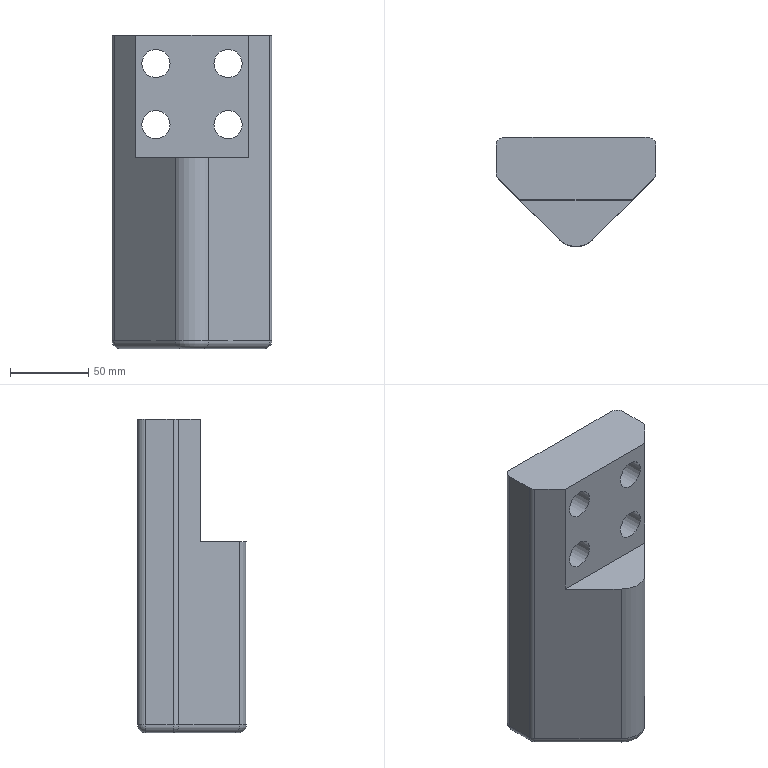Part | NX | features UB-7 2 | 1 solid | 36 faces | box 102 x 69.645 x 200 mm | volume 855541 mm3 | cylinder 18 | plane 13 | sphere 4 | torus 1 | commonest cylinder face diameters 10 x9 18 x4 26 x4 30 x1
STEP:
#1=CARTESIAN_POINT('',(3357.129,-625.444,973.716));
#2=VERTEX_POINT('',#1);
#3=CARTESIAN_POINT('',(3343.452,-639.122,973.716));
#4=VERTEX_POINT('',#3);
#5=CARTESIAN_POINT('',(3333.023,-649.551,973.716));
#6=DIRECTION('',(-0.7071,-0.7071,0.));
#7=VECTOR('',#6,1000.);
#8=LINE('',#5,#7);
#9=EDGE_CURVE('',#2,#4,#8,.T.);
#10=ORIENTED_EDGE('',*,*,#9,.F.);
#11=CARTESIAN_POINT('',(3358.594,-621.909,973.716));
#12=VERTEX_POINT('',#11);
#13=CARTESIAN_POINT('',(3353.594,-621.909,973.716));
#14=DIRECTION('',(0.,0.,-1.));
#15=DIRECTION('',(1.,0.,0.));
#16=AXIS2_PLACEMENT_3D('',#13,#14,#15);
#17=CIRCLE('',#16,5.);
#18=EDGE_CURVE('',#12,#2,#17,.T.);
#19=ORIENTED_EDGE('',*,*,#18,.F.);
#20=CARTESIAN_POINT('',(3358.594,-604.122,973.716));
#21=VERTEX_POINT('',#20);
#22=CARTESIAN_POINT('',(3358.594,-656.622,973.716));
#23=DIRECTION('',(0.,-1.,0.));
#24=VECTOR('',#23,1000.);
#25=LINE('',#22,#24);
#26=EDGE_CURVE('',#21,#12,#25,.T.);
#27=ORIENTED_EDGE('',*,*,#26,.F.);
#28=CARTESIAN_POINT('',(3353.594,-599.122,973.716));
#29=VERTEX_POINT('',#28);
#30=CARTESIAN_POINT('',(3353.594,-604.122,973.716));
#31=DIRECTION('',(0.,0.,-1.));
#32=DIRECTION('',(1.,0.,0.));
#33=AXIS2_PLACEMENT_3D('',#30,#31,#32);
#34=CIRCLE('',#33,5.);
#35=EDGE_CURVE('',#29,#21,#34,.T.);
#36=ORIENTED_EDGE('',*,*,#35,.F.);
#37=CARTESIAN_POINT('',(3331.979,-599.122,973.716));
#38=VERTEX_POINT('',#37);
#39=CARTESIAN_POINT('',(3325.523,-599.122,973.716));
#40=DIRECTION('',(-1.,0.,0.));
#41=VECTOR('',#40,1000.);
#42=LINE('',#39,#41);
#43=EDGE_CURVE('',#29,#38,#42,.T.);
#44=ORIENTED_EDGE('',*,*,#43,.T.);
#45=CARTESIAN_POINT('',(3261.594,-599.122,973.716));
#46=VERTEX_POINT('',#45);
#47=CARTESIAN_POINT('',(3325.523,-599.122,973.716));
#48=DIRECTION('',(-1.,0.,0.));
#49=VECTOR('',#48,1000.);
#50=LINE('',#47,#49);
#51=EDGE_CURVE('',#38,#46,#50,.T.);
#52=ORIENTED_EDGE('',*,*,#51,.T.);
#53=CARTESIAN_POINT('',(3256.594,-604.122,973.716));
#54=VERTEX_POINT('',#53);
#55=CARTESIAN_POINT('',(3261.594,-604.122,973.716));
#56=DIRECTION('',(0.,0.,-1.));
#57=DIRECTION('',(1.,0.,0.));
#58=AXIS2_PLACEMENT_3D('',#55,#56,#57);
#59=CIRCLE('',#58,5.);
#60=EDGE_CURVE('',#54,#46,#59,.T.);
#61=ORIENTED_EDGE('',*,*,#60,.F.);
#62=CARTESIAN_POINT('',(3256.594,-621.909,973.716));
#63=VERTEX_POINT('',#62);
#64=CARTESIAN_POINT('',(3256.594,-656.622,973.716));
#65=DIRECTION('',(0.,-1.,0.));
#66=VECTOR('',#65,1000.);
#67=LINE('',#64,#66);
#68=EDGE_CURVE('',#54,#63,#67,.T.);
#69=ORIENTED_EDGE('',*,*,#68,.T.);
#70=CARTESIAN_POINT('',(3258.058,-625.444,973.716));
#71=VERTEX_POINT('',#70);
#72=CARTESIAN_POINT('',(3261.594,-621.909,973.716));
#73=DIRECTION('',(0.,0.,-1.));
#74=DIRECTION('',(1.,0.,0.));
#75=AXIS2_PLACEMENT_3D('',#72,#73,#74);
#76=CIRCLE('',#75,5.);
#77=EDGE_CURVE('',#71,#63,#76,.T.);
#78=ORIENTED_EDGE('',*,*,#77,.F.);
#79=CARTESIAN_POINT('',(3271.736,-639.122,973.716));
#80=VERTEX_POINT('',#79);
#81=CARTESIAN_POINT('',(3297.165,-664.551,973.716));
#82=DIRECTION('',(0.7071,-0.7071,0.));
#83=VECTOR('',#82,1000.);
#84=LINE('',#81,#83);
#85=EDGE_CURVE('',#71,#80,#84,.T.);
#86=ORIENTED_EDGE('',*,*,#85,.T.);
#87=CARTESIAN_POINT('',(3307.594,-639.122,973.716));
#88=DIRECTION('',(1.,0.,0.));
#89=VECTOR('',#88,1000.);
#90=LINE('',#87,#89);
#91=EDGE_CURVE('',#80,#4,#90,.T.);
#92=ORIENTED_EDGE('',*,*,#91,.T.);
#93=EDGE_LOOP('',(#10,#19,#27,#36,#44,#52,#61,#69,#78,#86,#92));
#94=FACE_BOUND('',#93,.T.);
#95=CARTESIAN_POINT('',(3325.523,-642.051,973.716));
#96=DIRECTION('',(0.,0.,1.));
#97=DIRECTION('',(0.7071,0.7071,0.));
#98=AXIS2_PLACEMENT_3D('',#95,#96,#97);
#99=PLANE('',#98);
#100=ADVANCED_FACE('',(#94),#99,.T.);
#101=CARTESIAN_POINT('',(3258.058,-625.444,778.716));
#102=VERTEX_POINT('',#101);
#103=CARTESIAN_POINT('',(3258.058,-625.444,583.116));
#104=DIRECTION('',(0.,0.,1.));
#105=VECTOR('',#104,1000.);
#106=LINE('',#103,#105);
#107=EDGE_CURVE('',#102,#71,#106,.T.);
#108=ORIENTED_EDGE('',*,*,#107,.T.);
#109=ORIENTED_EDGE('',*,*,#77,.T.);
#110=CARTESIAN_POINT('',(3256.594,-621.909,778.716));
#111=VERTEX_POINT('',#110);
#112=CARTESIAN_POINT('',(3256.594,-621.909,938.716));
#113=DIRECTION('',(0.,0.,-1.));
#114=VECTOR('',#113,1000.);
#115=LINE('',#112,#114);
#116=EDGE_CURVE('',#63,#111,#115,.T.);
#117=ORIENTED_EDGE('',*,*,#116,.T.);
#118=CARTESIAN_POINT('',(3261.594,-621.909,778.716));
#119=DIRECTION('',(0.,0.,-1.));
#120=DIRECTION('',(1.,0.,0.));
#121=AXIS2_PLACEMENT_3D('',#118,#119,#120);
#122=CIRCLE('',#121,5.);
#123=EDGE_CURVE('',#102,#111,#122,.T.);
#124=ORIENTED_EDGE('',*,*,#123,.F.);
#125=EDGE_LOOP('',(#108,#109,#117,#124));
#126=FACE_BOUND('',#125,.T.);
#127=CARTESIAN_POINT('',(3261.594,-621.909,583.116));
#128=DIRECTION('',(0.,0.,1.));
#129=DIRECTION('',(-1.,0.,0.));
#130=AXIS2_PLACEMENT_3D('',#127,#128,#129);
#131=CYLINDRICAL_SURFACE('',#130,5.);
#132=ADVANCED_FACE('',(#126),#131,.T.);
#133=CARTESIAN_POINT('',(3358.594,-621.909,778.716));
#134=VERTEX_POINT('',#133);
#135=CARTESIAN_POINT('',(3358.594,-621.909,968.716));
#136=DIRECTION('',(0.,0.,1.));
#137=VECTOR('',#136,1000.);
#138=LINE('',#135,#137);
#139=EDGE_CURVE('',#134,#12,#138,.T.);
#140=ORIENTED_EDGE('',*,*,#139,.T.);
#141=ORIENTED_EDGE('',*,*,#18,.T.);
#142=CARTESIAN_POINT('',(3357.129,-625.444,778.716));
#143=VERTEX_POINT('',#142);
#144=CARTESIAN_POINT('',(3357.129,-625.444,943.716));
#145=DIRECTION('',(0.,0.,-1.));
#146=VECTOR('',#145,1000.);
#147=LINE('',#144,#146);
#148=EDGE_CURVE('',#2,#143,#147,.T.);
#149=ORIENTED_EDGE('',*,*,#148,.T.);
#150=CARTESIAN_POINT('',(3353.594,-621.909,778.716));
#151=DIRECTION('',(0.,0.,-1.));
#152=DIRECTION('',(1.,0.,0.));
#153=AXIS2_PLACEMENT_3D('',#150,#151,#152);
#154=CIRCLE('',#153,5.);
#155=EDGE_CURVE('',#134,#143,#154,.T.);
#156=ORIENTED_EDGE('',*,*,#155,.F.);
#157=EDGE_LOOP('',(#140,#141,#149,#156));
#158=FACE_BOUND('',#157,.T.);
#159=CARTESIAN_POINT('',(3353.594,-621.909,943.716));
#160=DIRECTION('',(0.,0.,1.));
#161=DIRECTION('',(-1.,0.,0.));
#162=AXIS2_PLACEMENT_3D('',#159,#160,#161);
#163=CYLINDRICAL_SURFACE('',#162,5.);
#164=ADVANCED_FACE('',(#158),#163,.T.);
#165=CARTESIAN_POINT('',(3353.594,-599.122,778.716));
#166=VERTEX_POINT('',#165);
#167=CARTESIAN_POINT('',(3353.594,-599.122,858.716));
#168=DIRECTION('',(0.,0.,1.));
#169=VECTOR('',#168,1000.);
#170=LINE('',#167,#169);
#171=EDGE_CURVE('',#166,#29,#170,.T.);
#172=ORIENTED_EDGE('',*,*,#171,.T.);
#173=ORIENTED_EDGE('',*,*,#35,.T.);
#174=CARTESIAN_POINT('',(3358.594,-604.122,778.716));
#175=VERTEX_POINT('',#174);
#176=CARTESIAN_POINT('',(3358.594,-604.122,938.716));
#177=DIRECTION('',(0.,0.,-1.));
#178=VECTOR('',#177,1000.);
#179=LINE('',#176,#178);
#180=EDGE_CURVE('',#21,#175,#179,.T.);
#181=ORIENTED_EDGE('',*,*,#180,.T.);
#182=CARTESIAN_POINT('',(3353.594,-604.122,778.716));
#183=DIRECTION('',(0.,0.,-1.));
#184=DIRECTION('',(1.,0.,0.));
#185=AXIS2_PLACEMENT_3D('',#182,#183,#184);
#186=CIRCLE('',#185,5.);
#187=EDGE_CURVE('',#166,#175,#186,.T.);
#188=ORIENTED_EDGE('',*,*,#187,.F.);
#189=EDGE_LOOP('',(#172,#173,#181,#188));
#190=FACE_BOUND('',#189,.T.);
#191=CARTESIAN_POINT('',(3353.594,-604.122,858.716));
#192=DIRECTION('',(0.,0.,1.));
#193=DIRECTION('',(-1.,0.,0.));
#194=AXIS2_PLACEMENT_3D('',#191,#192,#193);
#195=CYLINDRICAL_SURFACE('',#194,5.);
#196=ADVANCED_FACE('',(#190),#195,.T.);
#197=ORIENTED_EDGE('',*,*,#180,.F.);
#198=ORIENTED_EDGE('',*,*,#26,.T.);
#199=ORIENTED_EDGE('',*,*,#139,.F.);
#200=CARTESIAN_POINT('',(3358.594,-621.909,778.716));
#201=DIRECTION('',(0.,-1.,0.));
#202=VECTOR('',#201,1000.);
#203=LINE('',#200,#202);
#204=EDGE_CURVE('',#175,#134,#203,.T.);
#205=ORIENTED_EDGE('',*,*,#204,.F.);
#206=EDGE_LOOP('',(#197,#198,#199,#205));
#207=FACE_BOUND('',#206,.T.);
#208=CARTESIAN_POINT('',(3358.594,-656.622,938.716));
#209=DIRECTION('',(1.,0.,0.));
#210=DIRECTION('',(0.,0.,1.));
#211=AXIS2_PLACEMENT_3D('',#208,#209,#210);
#212=PLANE('',#211);
#213=ADVANCED_FACE('',(#207),#212,.T.);
#214=CARTESIAN_POINT('',(3256.594,-604.122,778.716));
#215=VERTEX_POINT('',#214);
#216=CARTESIAN_POINT('',(3256.594,-604.122,968.716));
#217=DIRECTION('',(0.,0.,1.));
#218=VECTOR('',#217,1000.);
#219=LINE('',#216,#218);
#220=EDGE_CURVE('',#215,#54,#219,.T.);
#221=ORIENTED_EDGE('',*,*,#220,.T.);
#222=ORIENTED_EDGE('',*,*,#60,.T.);
#223=CARTESIAN_POINT('',(3261.594,-599.122,778.716));
#224=VERTEX_POINT('',#223);
#225=CARTESIAN_POINT('',(3261.594,-599.122,898.716));
#226=DIRECTION('',(0.,0.,-1.));
#227=VECTOR('',#226,1000.);
#228=LINE('',#225,#227);
#229=EDGE_CURVE('',#46,#224,#228,.T.);
#230=ORIENTED_EDGE('',*,*,#229,.T.);
#231=CARTESIAN_POINT('',(3261.594,-604.122,778.716));
#232=DIRECTION('',(0.,0.,-1.));
#233=DIRECTION('',(-1.,0.,0.));
#234=AXIS2_PLACEMENT_3D('',#231,#232,#233);
#235=CIRCLE('',#234,5.);
#236=EDGE_CURVE('',#215,#224,#235,.T.);
#237=ORIENTED_EDGE('',*,*,#236,.F.);
#238=EDGE_LOOP('',(#221,#222,#230,#237));
#239=FACE_BOUND('',#238,.T.);
#240=CARTESIAN_POINT('',(3261.594,-604.122,858.716));
#241=DIRECTION('',(0.,0.,-1.));
#242=DIRECTION('',(1.,0.,0.));
#243=AXIS2_PLACEMENT_3D('',#240,#241,#242);
#244=CYLINDRICAL_SURFACE('',#243,5.);
#245=ADVANCED_FACE('',(#239),#244,.T.);
#246=CARTESIAN_POINT('',(3297.594,-599.122,955.716));
#247=VERTEX_POINT('',#246);
#248=CARTESIAN_POINT('',(3284.594,-599.122,955.716));
#249=DIRECTION('',(0.,-1.,0.));
#250=DIRECTION('',(1.,0.,0.));
#251=AXIS2_PLACEMENT_3D('',#248,#249,#250);
#252=CIRCLE('',#251,13.);
#253=EDGE_CURVE('',#247,#247,#252,.T.);
#254=ORIENTED_EDGE('',*,*,#253,.T.);
#255=EDGE_LOOP('',(#254));
#256=FACE_BOUND('',#255,.T.);
#257=CARTESIAN_POINT('',(3343.594,-599.122,916.716));
#258=VERTEX_POINT('',#257);
#259=CARTESIAN_POINT('',(3330.594,-599.122,916.716));
#260=DIRECTION('',(0.,-1.,0.));
#261=DIRECTION('',(1.,0.,0.));
#262=AXIS2_PLACEMENT_3D('',#259,#260,#261);
#263=CIRCLE('',#262,13.);
#264=EDGE_CURVE('',#258,#258,#263,.T.);
#265=ORIENTED_EDGE('',*,*,#264,.T.);
#266=EDGE_LOOP('',(#265));
#267=FACE_BOUND('',#266,.T.);
#268=CARTESIAN_POINT('',(3297.594,-599.122,916.716));
#269=VERTEX_POINT('',#268);
#270=CARTESIAN_POINT('',(3284.594,-599.122,916.716));
#271=DIRECTION('',(0.,-1.,0.));
#272=DIRECTION('',(1.,0.,0.));
#273=AXIS2_PLACEMENT_3D('',#270,#271,#272);
#274=CIRCLE('',#273,13.);
#275=EDGE_CURVE('',#269,#269,#274,.T.);
#276=ORIENTED_EDGE('',*,*,#275,.T.);
#277=EDGE_LOOP('',(#276));
#278=FACE_BOUND('',#277,.T.);
#279=CARTESIAN_POINT('',(3343.594,-599.122,955.716));
#280=VERTEX_POINT('',#279);
#281=CARTESIAN_POINT('',(3330.594,-599.122,955.716));
#282=DIRECTION('',(0.,-1.,0.));
#283=DIRECTION('',(1.,0.,0.));
#284=AXIS2_PLACEMENT_3D('',#281,#282,#283);
#285=CIRCLE('',#284,13.);
#286=EDGE_CURVE('',#280,#280,#285,.T.);
#287=ORIENTED_EDGE('',*,*,#286,.T.);
#288=EDGE_LOOP('',(#287));
#289=FACE_BOUND('',#288,.T.);
#290=ORIENTED_EDGE('',*,*,#229,.F.);
#291=ORIENTED_EDGE('',*,*,#51,.F.);
#292=ORIENTED_EDGE('',*,*,#43,.F.);
#293=ORIENTED_EDGE('',*,*,#171,.F.);
#294=CARTESIAN_POINT('',(3353.594,-599.122,778.716));
#295=DIRECTION('',(1.,0.,0.));
#296=VECTOR('',#295,1000.);
#297=LINE('',#294,#296);
#298=EDGE_CURVE('',#224,#166,#297,.T.);
#299=ORIENTED_EDGE('',*,*,#298,.F.);
#300=EDGE_LOOP('',(#290,#291,#292,#293,#299));
#301=FACE_BOUND('',#300,.T.);
#302=CARTESIAN_POINT('',(4400.094,-599.122,858.716));
#303=DIRECTION('',(0.,1.,0.));
#304=DIRECTION('',(-1.,0.,0.));
#305=AXIS2_PLACEMENT_3D('',#302,#303,#304);
#306=PLANE('',#305);
#307=ADVANCED_FACE('',(#256,#267,#278,#289,#301),#306,.T.);
#308=CARTESIAN_POINT('',(3293.594,-639.122,955.716));
#309=VERTEX_POINT('',#308);
#310=CARTESIAN_POINT('',(3284.594,-639.122,955.716));
#311=DIRECTION('',(0.,-1.,0.));
#312=DIRECTION('',(1.,0.,0.));
#313=AXIS2_PLACEMENT_3D('',#310,#311,#312);
#314=CIRCLE('',#313,9.);
#315=EDGE_CURVE('',#309,#309,#314,.T.);
#316=ORIENTED_EDGE('',*,*,#315,.F.);
#317=EDGE_LOOP('',(#316));
#318=FACE_BOUND('',#317,.T.);
#319=CARTESIAN_POINT('',(3339.594,-639.122,916.716));
#320=VERTEX_POINT('',#319);
#321=CARTESIAN_POINT('',(3330.594,-639.122,916.716));
#322=DIRECTION('',(0.,-1.,0.));
#323=DIRECTION('',(1.,0.,0.));
#324=AXIS2_PLACEMENT_3D('',#321,#322,#323);
#325=CIRCLE('',#324,9.);
#326=EDGE_CURVE('',#320,#320,#325,.T.);
#327=ORIENTED_EDGE('',*,*,#326,.F.);
#328=EDGE_LOOP('',(#327));
#329=FACE_BOUND('',#328,.T.);
#330=CARTESIAN_POINT('',(3293.594,-639.122,916.716));
#331=VERTEX_POINT('',#330);
#332=CARTESIAN_POINT('',(3284.594,-639.122,916.716));
#333=DIRECTION('',(0.,-1.,0.));
#334=DIRECTION('',(1.,0.,0.));
#335=AXIS2_PLACEMENT_3D('',#332,#333,#334);
#336=CIRCLE('',#335,9.);
#337=EDGE_CURVE('',#331,#331,#336,.T.);
#338=ORIENTED_EDGE('',*,*,#337,.F.);
#339=EDGE_LOOP('',(#338));
#340=FACE_BOUND('',#339,.T.);
#341=CARTESIAN_POINT('',(3339.594,-639.122,955.716));
#342=VERTEX_POINT('',#341);
#343=CARTESIAN_POINT('',(3330.594,-639.122,955.716));
#344=DIRECTION('',(0.,-1.,0.));
#345=DIRECTION('',(1.,0.,0.));
#346=AXIS2_PLACEMENT_3D('',#343,#344,#345);
#347=CIRCLE('',#346,9.);
#348=EDGE_CURVE('',#342,#342,#347,.T.);
#349=ORIENTED_EDGE('',*,*,#348,.F.);
#350=EDGE_LOOP('',(#349));
#351=FACE_BOUND('',#350,.T.);
#352=CARTESIAN_POINT('',(3343.452,-639.122,895.716));
#353=VERTEX_POINT('',#352);
#354=CARTESIAN_POINT('',(3343.452,-639.122,943.716));
#355=DIRECTION('',(0.,0.,1.));
#356=VECTOR('',#355,1000.);
#357=LINE('',#354,#356);
#358=EDGE_CURVE('',#353,#4,#357,.T.);
#359=ORIENTED_EDGE('',*,*,#358,.T.);
#360=ORIENTED_EDGE('',*,*,#91,.F.);
#361=CARTESIAN_POINT('',(3271.736,-639.122,895.716));
#362=VERTEX_POINT('',#361);
#363=CARTESIAN_POINT('',(3271.736,-639.122,933.716));
#364=DIRECTION('',(0.,0.,1.));
#365=VECTOR('',#364,1000.);
#366=LINE('',#363,#365);
#367=EDGE_CURVE('',#362,#80,#366,.T.);
#368=ORIENTED_EDGE('',*,*,#367,.F.);
#369=CARTESIAN_POINT('',(3307.594,-639.122,895.716));
#370=DIRECTION('',(-1.,0.,0.));
#371=VECTOR('',#370,1000.);
#372=LINE('',#369,#371);
#373=EDGE_CURVE('',#353,#362,#372,.T.);
#374=ORIENTED_EDGE('',*,*,#373,.F.);
#375=EDGE_LOOP('',(#359,#360,#368,#374));
#376=FACE_BOUND('',#375,.T.);
#377=CARTESIAN_POINT('',(3307.594,-639.122,933.716));
#378=DIRECTION('',(0.,1.,0.));
#379=DIRECTION('',(-1.,0.,0.));
#380=AXIS2_PLACEMENT_3D('',#377,#378,#379);
#381=PLANE('',#380);
#382=ADVANCED_FACE('',(#318,#329,#340,#351,#376),#381,.F.);
#383=ORIENTED_EDGE('',*,*,#148,.F.);
#384=ORIENTED_EDGE('',*,*,#9,.T.);
#385=ORIENTED_EDGE('',*,*,#358,.F.);
#386=CARTESIAN_POINT('',(3318.201,-664.373,895.716));
#387=VERTEX_POINT('',#386);
#388=CARTESIAN_POINT('',(3333.023,-649.551,895.716));
#389=DIRECTION('',(0.7071,0.7071,0.));
#390=VECTOR('',#389,1000.);
#391=LINE('',#388,#390);
#392=EDGE_CURVE('',#387,#353,#391,.T.);
#393=ORIENTED_EDGE('',*,*,#392,.F.);
#394=CARTESIAN_POINT('',(3318.201,-664.373,778.716));
#395=VERTEX_POINT('',#394);
#396=CARTESIAN_POINT('',(3318.201,-664.373,943.716));
#397=DIRECTION('',(0.,0.,1.));
#398=VECTOR('',#397,1000.);
#399=LINE('',#396,#398);
#400=EDGE_CURVE('',#395,#387,#399,.T.);
#401=ORIENTED_EDGE('',*,*,#400,.F.);
#402=CARTESIAN_POINT('',(3333.023,-649.551,778.716));
#403=DIRECTION('',(-0.7071,-0.7071,0.));
#404=VECTOR('',#403,1000.);
#405=LINE('',#402,#404);
#406=EDGE_CURVE('',#143,#395,#405,.T.);
#407=ORIENTED_EDGE('',*,*,#406,.F.);
#408=EDGE_LOOP('',(#383,#384,#385,#393,#401,#407));
#409=FACE_BOUND('',#408,.T.);
#410=CARTESIAN_POINT('',(3333.023,-649.551,943.716));
#411=DIRECTION('',(-0.7071,0.7071,0.));
#412=DIRECTION('',(-0.7071,-0.7071,0.));
#413=AXIS2_PLACEMENT_3D('',#410,#411,#412);
#414=PLANE('',#413);
#415=ADVANCED_FACE('',(#409),#414,.F.);
#416=ORIENTED_EDGE('',*,*,#116,.F.);
#417=ORIENTED_EDGE('',*,*,#68,.F.);
#418=ORIENTED_EDGE('',*,*,#220,.F.);
#419=CARTESIAN_POINT('',(3256.594,-656.622,778.716));
#420=DIRECTION('',(0.,1.,0.));
#421=VECTOR('',#420,1000.);
#422=LINE('',#419,#421);
#423=EDGE_CURVE('',#111,#215,#422,.T.);
#424=ORIENTED_EDGE('',*,*,#423,.F.);
#425=EDGE_LOOP('',(#416,#417,#418,#424));
#426=FACE_BOUND('',#425,.T.);
#427=CARTESIAN_POINT('',(3256.594,-656.622,938.716));
#428=DIRECTION('',(-1.,0.,0.));
#429=DIRECTION('',(0.,0.,-1.));
#430=AXIS2_PLACEMENT_3D('',#427,#428,#429);
#431=PLANE('',#430);
#432=ADVANCED_FACE('',(#426),#431,.T.);
#433=ORIENTED_EDGE('',*,*,#367,.T.);
#434=ORIENTED_EDGE('',*,*,#85,.F.);
#435=ORIENTED_EDGE('',*,*,#107,.F.);
#436=CARTESIAN_POINT('',(3296.987,-664.373,778.716));
#437=VERTEX_POINT('',#436);
#438=CARTESIAN_POINT('',(3297.165,-664.551,778.716));
#439=DIRECTION('',(-0.7071,0.7071,0.));
#440=VECTOR('',#439,1000.);
#441=LINE('',#438,#440);
#442=EDGE_CURVE('',#437,#102,#441,.T.);
#443=ORIENTED_EDGE('',*,*,#442,.F.);
#444=CARTESIAN_POINT('',(3296.987,-664.373,895.716));
#445=VERTEX_POINT('',#444);
#446=CARTESIAN_POINT('',(3296.987,-664.373,583.116));
#447=DIRECTION('',(0.,0.,-1.));
#448=VECTOR('',#447,1000.);
#449=LINE('',#446,#448);
#450=EDGE_CURVE('',#445,#437,#449,.T.);
#451=ORIENTED_EDGE('',*,*,#450,.F.);
#452=CARTESIAN_POINT('',(3297.165,-664.551,895.716));
#453=DIRECTION('',(0.7071,-0.7071,0.));
#454=VECTOR('',#453,1000.);
#455=LINE('',#452,#454);
#456=EDGE_CURVE('',#362,#445,#455,.T.);
#457=ORIENTED_EDGE('',*,*,#456,.F.);
#458=EDGE_LOOP('',(#433,#434,#435,#443,#451,#457));
#459=FACE_BOUND('',#458,.T.);
#460=CARTESIAN_POINT('',(3297.165,-664.551,583.116));
#461=DIRECTION('',(-0.7071,-0.7071,0.));
#462=DIRECTION('',(0.,0.,1.));
#463=AXIS2_PLACEMENT_3D('',#460,#461,#462);
#464=PLANE('',#463);
#465=ADVANCED_FACE('',(#459),#464,.T.);
#466=ORIENTED_EDGE('',*,*,#392,.T.);
#467=ORIENTED_EDGE('',*,*,#373,.T.);
#468=ORIENTED_EDGE('',*,*,#456,.T.);
#469=CARTESIAN_POINT('',(3307.594,-653.767,895.716));
#470=DIRECTION('',(0.,0.,-1.));
#471=DIRECTION('',(-1.,0.,0.));
#472=AXIS2_PLACEMENT_3D('',#469,#470,#471);
#473=CIRCLE('',#472,15.);
#474=EDGE_CURVE('',#387,#445,#473,.T.);
#475=ORIENTED_EDGE('',*,*,#474,.F.);
#476=EDGE_LOOP('',(#466,#467,#468,#475));
#477=FACE_BOUND('',#476,.T.);
#478=CARTESIAN_POINT('',(3307.594,-651.622,895.716));
#479=DIRECTION('',(0.,0.,-1.));
#480=DIRECTION('',(1.,0.,0.));
#481=AXIS2_PLACEMENT_3D('',#478,#479,#480);
#482=PLANE('',#481);
#483=ADVANCED_FACE('',(#477),#482,.F.);
#484=CARTESIAN_POINT('',(3314.665,-660.838,773.716));
#485=VERTEX_POINT('',#484);
#486=CARTESIAN_POINT('',(3353.594,-621.909,773.716));
#487=VERTEX_POINT('',#486);
#488=CARTESIAN_POINT('',(3329.487,-646.015,773.716));
#489=DIRECTION('',(0.7071,0.7071,0.));
#490=VECTOR('',#489,1000.);
#491=LINE('',#488,#490);
#492=EDGE_CURVE('',#485,#487,#491,.T.);
#493=ORIENTED_EDGE('',*,*,#492,.F.);
#494=CARTESIAN_POINT('',(3300.523,-660.838,773.716));
#495=VERTEX_POINT('',#494);
#496=CARTESIAN_POINT('',(3307.594,-653.767,773.716));
#497=DIRECTION('',(0.,0.,1.));
#498=DIRECTION('',(1.,0.,0.));
#499=AXIS2_PLACEMENT_3D('',#496,#497,#498);
#500=CIRCLE('',#499,10.);
#501=EDGE_CURVE('',#495,#485,#500,.T.);
#502=ORIENTED_EDGE('',*,*,#501,.F.);
#503=CARTESIAN_POINT('',(3261.594,-621.909,773.716));
#504=VERTEX_POINT('',#503);
#505=CARTESIAN_POINT('',(3303.629,-663.944,773.716));
#506=DIRECTION('',(0.7071,-0.7071,0.));
#507=VECTOR('',#506,1000.);
#508=LINE('',#505,#507);
#509=EDGE_CURVE('',#504,#495,#508,.T.);
#510=ORIENTED_EDGE('',*,*,#509,.F.);
#511=CARTESIAN_POINT('',(3261.594,-604.122,773.716));
#512=VERTEX_POINT('',#511);
#513=CARTESIAN_POINT('',(3261.594,-642.051,773.716));
#514=DIRECTION('',(0.,-1.,0.));
#515=VECTOR('',#514,1000.);
#516=LINE('',#513,#515);
#517=EDGE_CURVE('',#512,#504,#516,.T.);
#518=ORIENTED_EDGE('',*,*,#517,.F.);
#519=CARTESIAN_POINT('',(3353.594,-604.122,773.716));
#520=VERTEX_POINT('',#519);
#521=CARTESIAN_POINT('',(3261.594,-604.122,773.716));
#522=DIRECTION('',(-1.,0.,0.));
#523=VECTOR('',#522,1000.);
#524=LINE('',#521,#523);
#525=EDGE_CURVE('',#520,#512,#524,.T.);
#526=ORIENTED_EDGE('',*,*,#525,.F.);
#527=CARTESIAN_POINT('',(3353.594,-609.122,773.716));
#528=DIRECTION('',(0.,1.,0.));
#529=VECTOR('',#528,1000.);
#530=LINE('',#527,#529);
#531=EDGE_CURVE('',#487,#520,#530,.T.);
#532=ORIENTED_EDGE('',*,*,#531,.F.);
#533=EDGE_LOOP('',(#493,#502,#510,#518,#526,#532));
#534=FACE_BOUND('',#533,.T.);
#535=CARTESIAN_POINT('',(3325.523,-642.051,773.716));
#536=DIRECTION('',(0.,0.,1.));
#537=DIRECTION('',(0.7071,0.7071,0.));
#538=AXIS2_PLACEMENT_3D('',#535,#536,#537);
#539=PLANE('',#538);
#540=ADVANCED_FACE('',(#534),#539,.F.);
#541=ORIENTED_EDGE('',*,*,#400,.T.);
#542=ORIENTED_EDGE('',*,*,#474,.T.);
#543=ORIENTED_EDGE('',*,*,#450,.T.);
#544=CARTESIAN_POINT('',(3307.594,-653.767,778.716));
#545=DIRECTION('',(0.,0.,-1.));
#546=DIRECTION('',(1.,0.,0.));
#547=AXIS2_PLACEMENT_3D('',#544,#545,#546);
#548=CIRCLE('',#547,15.);
#549=EDGE_CURVE('',#395,#437,#548,.T.);
#550=ORIENTED_EDGE('',*,*,#549,.F.);
#551=EDGE_LOOP('',(#541,#542,#543,#550));
#552=FACE_BOUND('',#551,.T.);
#553=CARTESIAN_POINT('',(3307.594,-653.767,583.116));
#554=DIRECTION('',(0.,0.,1.));
#555=DIRECTION('',(-1.,0.,0.));
#556=AXIS2_PLACEMENT_3D('',#553,#554,#555);
#557=CYLINDRICAL_SURFACE('',#556,15.);
#558=ADVANCED_FACE('',(#552),#557,.T.);
#559=CARTESIAN_POINT('',(3261.594,-621.909,778.716));
#560=DIRECTION('',(0.,-1.,0.));
#561=DIRECTION('',(0.,0.,-1.));
#562=AXIS2_PLACEMENT_3D('',#559,#560,#561);
#563=CIRCLE('',#562,5.);
#564=EDGE_CURVE('',#111,#504,#563,.T.);
#565=ORIENTED_EDGE('',*,*,#564,.T.);
#566=CARTESIAN_POINT('',(3261.594,-621.909,778.716));
#567=DIRECTION('',(-0.7071,0.7071,0.));
#568=DIRECTION('',(-0.7071,-0.7071,0.));
#569=AXIS2_PLACEMENT_3D('',#566,#567,#568);
#570=CIRCLE('',#569,5.);
#571=EDGE_CURVE('',#504,#102,#570,.T.);
#572=ORIENTED_EDGE('',*,*,#571,.T.);
#573=ORIENTED_EDGE('',*,*,#123,.T.);
#574=EDGE_LOOP('',(#565,#572,#573));
#575=FACE_BOUND('',#574,.T.);
#576=CARTESIAN_POINT('',(3261.594,-621.909,778.716));
#577=DIRECTION('',(0.,0.,1.));
#578=DIRECTION('',(-1.,0.,0.));
#579=AXIS2_PLACEMENT_3D('',#576,#577,#578);
#580=SPHERICAL_SURFACE('',#579,5.);
#581=ADVANCED_FACE('',(#575),#580,.T.);
#582=ORIENTED_EDGE('',*,*,#571,.F.);
#583=ORIENTED_EDGE('',*,*,#509,.T.);
#584=CARTESIAN_POINT('',(3300.523,-660.838,778.716));
#585=DIRECTION('',(-0.7071,0.7071,0.));
#586=DIRECTION('',(-0.7071,-0.7071,0.));
#587=AXIS2_PLACEMENT_3D('',#584,#585,#586);
#588=CIRCLE('',#587,5.);
#589=EDGE_CURVE('',#495,#437,#588,.T.);
#590=ORIENTED_EDGE('',*,*,#589,.T.);
#591=ORIENTED_EDGE('',*,*,#442,.T.);
#592=EDGE_LOOP('',(#582,#583,#590,#591));
#593=FACE_BOUND('',#592,.T.);
#594=CARTESIAN_POINT('',(3300.701,-661.015,778.716));
#595=DIRECTION('',(0.7071,-0.7071,0.));
#596=DIRECTION('',(0.7071,0.7071,0.));
#597=AXIS2_PLACEMENT_3D('',#594,#595,#596);
#598=CYLINDRICAL_SURFACE('',#597,5.);
#599=ADVANCED_FACE('',(#593),#598,.T.);
#600=ORIENTED_EDGE('',*,*,#564,.F.);
#601=ORIENTED_EDGE('',*,*,#423,.T.);
#602=CARTESIAN_POINT('',(3261.594,-604.122,778.716));
#603=DIRECTION('',(0.,-1.,0.));
#604=DIRECTION('',(0.,0.,-1.));
#605=AXIS2_PLACEMENT_3D('',#602,#603,#604);
#606=CIRCLE('',#605,5.);
#607=EDGE_CURVE('',#215,#512,#606,.T.);
#608=ORIENTED_EDGE('',*,*,#607,.T.);
#609=ORIENTED_EDGE('',*,*,#517,.T.);
#610=EDGE_LOOP('',(#600,#601,#608,#609));
#611=FACE_BOUND('',#610,.T.);
#612=CARTESIAN_POINT('',(3261.594,-642.051,778.716));
#613=DIRECTION('',(0.,1.,0.));
#614=DIRECTION('',(0.,0.,1.));
#615=AXIS2_PLACEMENT_3D('',#612,#613,#614);
#616=CYLINDRICAL_SURFACE('',#615,5.);
#617=ADVANCED_FACE('',(#611),#616,.T.);
#618=ORIENTED_EDGE('',*,*,#589,.F.);
#619=ORIENTED_EDGE('',*,*,#501,.T.);
#620=CARTESIAN_POINT('',(3314.665,-660.838,778.716));
#621=DIRECTION('',(-0.7071,-0.7071,0.));
#622=DIRECTION('',(-0.7071,0.7071,0.));
#623=AXIS2_PLACEMENT_3D('',#620,#621,#622);
#624=CIRCLE('',#623,5.);
#625=EDGE_CURVE('',#485,#395,#624,.T.);
#626=ORIENTED_EDGE('',*,*,#625,.T.);
#627=ORIENTED_EDGE('',*,*,#549,.T.);
#628=EDGE_LOOP('',(#618,#619,#626,#627));
#629=FACE_BOUND('',#628,.T.);
#630=CARTESIAN_POINT('',(3307.594,-653.767,778.716));
#631=DIRECTION('',(0.,0.,1.));
#632=DIRECTION('',(-1.,0.,0.));
#633=AXIS2_PLACEMENT_3D('',#630,#631,#632);
#634=TOROIDAL_SURFACE('',#633,10.,5.);
#635=ADVANCED_FACE('',(#629),#634,.T.);
#636=ORIENTED_EDGE('',*,*,#236,.T.);
#637=CARTESIAN_POINT('',(3261.594,-604.122,778.716));
#638=DIRECTION('',(-1.,0.,0.));
#639=DIRECTION('',(0.,-1.,0.));
#640=AXIS2_PLACEMENT_3D('',#637,#638,#639);
#641=CIRCLE('',#640,5.);
#642=EDGE_CURVE('',#224,#512,#641,.T.);
#643=ORIENTED_EDGE('',*,*,#642,.T.);
#644=ORIENTED_EDGE('',*,*,#607,.F.);
#645=EDGE_LOOP('',(#636,#643,#644));
#646=FACE_BOUND('',#645,.T.);
#647=CARTESIAN_POINT('',(3261.594,-604.122,778.716));
#648=DIRECTION('',(0.,0.,1.));
#649=DIRECTION('',(-1.,0.,0.));
#650=AXIS2_PLACEMENT_3D('',#647,#648,#649);
#651=SPHERICAL_SURFACE('',#650,5.);
#652=ADVANCED_FACE('',(#646),#651,.T.);
#653=ORIENTED_EDGE('',*,*,#625,.F.);
#654=ORIENTED_EDGE('',*,*,#492,.T.);
#655=CARTESIAN_POINT('',(3353.594,-621.909,778.716));
#656=DIRECTION('',(-0.7071,-0.7071,0.));
#657=DIRECTION('',(-0.7071,0.7071,0.));
#658=AXIS2_PLACEMENT_3D('',#655,#656,#657);
#659=CIRCLE('',#658,5.);
#660=EDGE_CURVE('',#487,#143,#659,.T.);
#661=ORIENTED_EDGE('',*,*,#660,.T.);
#662=ORIENTED_EDGE('',*,*,#406,.T.);
#663=EDGE_LOOP('',(#653,#654,#661,#662));
#664=FACE_BOUND('',#663,.T.);
#665=CARTESIAN_POINT('',(3329.487,-646.015,778.716));
#666=DIRECTION('',(-0.7071,-0.7071,0.));
#667=DIRECTION('',(0.7071,-0.7071,0.));
#668=AXIS2_PLACEMENT_3D('',#665,#666,#667);
#669=CYLINDRICAL_SURFACE('',#668,5.);
#670=ADVANCED_FACE('',(#664),#669,.T.);
#671=ORIENTED_EDGE('',*,*,#642,.F.);
#672=ORIENTED_EDGE('',*,*,#298,.T.);
#673=CARTESIAN_POINT('',(3353.594,-604.122,778.716));
#674=DIRECTION('',(-1.,0.,0.));
#675=DIRECTION('',(0.,-1.,0.));
#676=AXIS2_PLACEMENT_3D('',#673,#674,#675);
#677=CIRCLE('',#676,5.);
#678=EDGE_CURVE('',#166,#520,#677,.T.);
#679=ORIENTED_EDGE('',*,*,#678,.T.);
#680=ORIENTED_EDGE('',*,*,#525,.T.);
#681=EDGE_LOOP('',(#671,#672,#679,#680));
#682=FACE_BOUND('',#681,.T.);
#683=CARTESIAN_POINT('',(3325.523,-604.122,778.716));
#684=DIRECTION('',(1.,0.,0.));
#685=DIRECTION('',(0.,1.,0.));
#686=AXIS2_PLACEMENT_3D('',#683,#684,#685);
#687=CYLINDRICAL_SURFACE('',#686,5.);
#688=ADVANCED_FACE('',(#682),#687,.T.);
#689=ORIENTED_EDGE('',*,*,#660,.F.);
#690=CARTESIAN_POINT('',(3353.594,-621.909,778.716));
#691=DIRECTION('',(0.,-1.,0.));
#692=DIRECTION('',(0.,0.,1.));
#693=AXIS2_PLACEMENT_3D('',#690,#691,#692);
#694=CIRCLE('',#693,5.);
#695=EDGE_CURVE('',#487,#134,#694,.T.);
#696=ORIENTED_EDGE('',*,*,#695,.T.);
#697=ORIENTED_EDGE('',*,*,#155,.T.);
#698=EDGE_LOOP('',(#689,#696,#697));
#699=FACE_BOUND('',#698,.T.);
#700=CARTESIAN_POINT('',(3353.594,-621.909,778.716));
#701=DIRECTION('',(0.,0.,1.));
#702=DIRECTION('',(-1.,0.,0.));
#703=AXIS2_PLACEMENT_3D('',#700,#701,#702);
#704=SPHERICAL_SURFACE('',#703,5.);
#705=ADVANCED_FACE('',(#699),#704,.T.);
#706=ORIENTED_EDGE('',*,*,#187,.T.);
#707=CARTESIAN_POINT('',(3353.594,-604.122,778.716));
#708=DIRECTION('',(0.,1.,0.));
#709=DIRECTION('',(0.,0.,1.));
#710=AXIS2_PLACEMENT_3D('',#707,#708,#709);
#711=CIRCLE('',#710,5.);
#712=EDGE_CURVE('',#175,#520,#711,.T.);
#713=ORIENTED_EDGE('',*,*,#712,.T.);
#714=ORIENTED_EDGE('',*,*,#678,.F.);
#715=EDGE_LOOP('',(#706,#713,#714));
#716=FACE_BOUND('',#715,.T.);
#717=CARTESIAN_POINT('',(3353.594,-604.122,778.716));
#718=DIRECTION('',(0.,0.,1.));
#719=DIRECTION('',(-1.,0.,0.));
#720=AXIS2_PLACEMENT_3D('',#717,#718,#719);
#721=SPHERICAL_SURFACE('',#720,5.);
#722=ADVANCED_FACE('',(#716),#721,.T.);
#723=ORIENTED_EDGE('',*,*,#695,.F.);
#724=ORIENTED_EDGE('',*,*,#531,.T.);
#725=ORIENTED_EDGE('',*,*,#712,.F.);
#726=ORIENTED_EDGE('',*,*,#204,.T.);
#727=EDGE_LOOP('',(#723,#724,#725,#726));
#728=FACE_BOUND('',#727,.T.);
#729=CARTESIAN_POINT('',(3353.594,-642.051,778.716));
#730=DIRECTION('',(0.,-1.,0.));
#731=DIRECTION('',(0.,0.,-1.));
#732=AXIS2_PLACEMENT_3D('',#729,#730,#731);
#733=CYLINDRICAL_SURFACE('',#732,5.);
#734=ADVANCED_FACE('',(#728),#733,.T.);
#735=CARTESIAN_POINT('',(3339.594,-618.122,955.716));
#736=VERTEX_POINT('',#735);
#737=CARTESIAN_POINT('',(3330.594,-618.122,955.716));
#738=DIRECTION('',(0.,-1.,0.));
#739=DIRECTION('',(1.,0.,0.));
#740=AXIS2_PLACEMENT_3D('',#737,#738,#739);
#741=CIRCLE('',#740,9.);
#742=EDGE_CURVE('',#736,#736,#741,.T.);
#743=ORIENTED_EDGE('',*,*,#742,.F.);
#744=EDGE_LOOP('',(#743));
#745=FACE_BOUND('',#744,.T.);
#746=ORIENTED_EDGE('',*,*,#348,.T.);
#747=EDGE_LOOP('',(#746));
#748=FACE_BOUND('',#747,.T.);
#749=CARTESIAN_POINT('',(3330.594,-640.122,955.716));
#750=DIRECTION('',(0.,1.,0.));
#751=DIRECTION('',(0.,0.,1.));
#752=AXIS2_PLACEMENT_3D('',#749,#750,#751);
#753=CYLINDRICAL_SURFACE('',#752,9.);
#754=ADVANCED_FACE('',(#745,#748),#753,.F.);
#755=ORIENTED_EDGE('',*,*,#286,.F.);
#756=EDGE_LOOP('',(#755));
#757=FACE_BOUND('',#756,.T.);
#758=CARTESIAN_POINT('',(3317.594,-618.122,955.716));
#759=VERTEX_POINT('',#758);
#760=CARTESIAN_POINT('',(3330.594,-618.122,955.716));
#761=DIRECTION('',(0.,1.,0.));
#762=DIRECTION('',(-1.,0.,0.));
#763=AXIS2_PLACEMENT_3D('',#760,#761,#762);
#764=CIRCLE('',#763,13.);
#765=EDGE_CURVE('',#759,#759,#764,.T.);
#766=ORIENTED_EDGE('',*,*,#765,.F.);
#767=EDGE_LOOP('',(#766));
#768=FACE_BOUND('',#767,.T.);
#769=CARTESIAN_POINT('',(3330.594,-618.122,955.716));
#770=DIRECTION('',(0.,1.,0.));
#771=DIRECTION('',(0.,0.,1.));
#772=AXIS2_PLACEMENT_3D('',#769,#770,#771);
#773=CYLINDRICAL_SURFACE('',#772,13.);
#774=ADVANCED_FACE('',(#757,#768),#773,.F.);
#775=ORIENTED_EDGE('',*,*,#742,.T.);
#776=EDGE_LOOP('',(#775));
#777=FACE_BOUND('',#776,.T.);
#778=ORIENTED_EDGE('',*,*,#765,.T.);
#779=EDGE_LOOP('',(#778));
#780=FACE_BOUND('',#779,.T.);
#781=CARTESIAN_POINT('',(3330.594,-618.122,955.716));
#782=DIRECTION('',(0.,1.,0.));
#783=DIRECTION('',(-1.,0.,0.));
#784=AXIS2_PLACEMENT_3D('',#781,#782,#783);
#785=PLANE('',#784);
#786=ADVANCED_FACE('',(#777,#780),#785,.T.);
#787=CARTESIAN_POINT('',(3293.594,-618.122,916.716));
#788=VERTEX_POINT('',#787);
#789=CARTESIAN_POINT('',(3284.594,-618.122,916.716));
#790=DIRECTION('',(0.,-1.,0.));
#791=DIRECTION('',(1.,0.,0.));
#792=AXIS2_PLACEMENT_3D('',#789,#790,#791);
#793=CIRCLE('',#792,9.);
#794=EDGE_CURVE('',#788,#788,#793,.T.);
#795=ORIENTED_EDGE('',*,*,#794,.F.);
#796=EDGE_LOOP('',(#795));
#797=FACE_BOUND('',#796,.T.);
#798=ORIENTED_EDGE('',*,*,#337,.T.);
#799=EDGE_LOOP('',(#798));
#800=FACE_BOUND('',#799,.T.);
#801=CARTESIAN_POINT('',(3284.594,-640.122,916.716));
#802=DIRECTION('',(0.,1.,0.));
#803=DIRECTION('',(0.,0.,1.));
#804=AXIS2_PLACEMENT_3D('',#801,#802,#803);
#805=CYLINDRICAL_SURFACE('',#804,9.);
#806=ADVANCED_FACE('',(#797,#800),#805,.F.);
#807=ORIENTED_EDGE('',*,*,#275,.F.);
#808=EDGE_LOOP('',(#807));
#809=FACE_BOUND('',#808,.T.);
#810=CARTESIAN_POINT('',(3271.594,-618.122,916.716));
#811=VERTEX_POINT('',#810);
#812=CARTESIAN_POINT('',(3284.594,-618.122,916.716));
#813=DIRECTION('',(0.,1.,0.));
#814=DIRECTION('',(-1.,0.,0.));
#815=AXIS2_PLACEMENT_3D('',#812,#813,#814);
#816=CIRCLE('',#815,13.);
#817=EDGE_CURVE('',#811,#811,#816,.T.);
#818=ORIENTED_EDGE('',*,*,#817,.F.);
#819=EDGE_LOOP('',(#818));
#820=FACE_BOUND('',#819,.T.);
#821=CARTESIAN_POINT('',(3284.594,-618.122,916.716));
#822=DIRECTION('',(0.,1.,0.));
#823=DIRECTION('',(0.,0.,1.));
#824=AXIS2_PLACEMENT_3D('',#821,#822,#823);
#825=CYLINDRICAL_SURFACE('',#824,13.);
#826=ADVANCED_FACE('',(#809,#820),#825,.F.);
#827=ORIENTED_EDGE('',*,*,#794,.T.);
#828=EDGE_LOOP('',(#827));
#829=FACE_BOUND('',#828,.T.);
#830=ORIENTED_EDGE('',*,*,#817,.T.);
#831=EDGE_LOOP('',(#830));
#832=FACE_BOUND('',#831,.T.);
#833=CARTESIAN_POINT('',(3284.594,-618.122,916.716));
#834=DIRECTION('',(0.,1.,0.));
#835=DIRECTION('',(-1.,0.,0.));
#836=AXIS2_PLACEMENT_3D('',#833,#834,#835);
#837=PLANE('',#836);
#838=ADVANCED_FACE('',(#829,#832),#837,.T.);
#839=CARTESIAN_POINT('',(3339.594,-618.122,916.716));
#840=VERTEX_POINT('',#839);
#841=CARTESIAN_POINT('',(3330.594,-618.122,916.716));
#842=DIRECTION('',(0.,-1.,0.));
#843=DIRECTION('',(1.,0.,0.));
#844=AXIS2_PLACEMENT_3D('',#841,#842,#843);
#845=CIRCLE('',#844,9.);
#846=EDGE_CURVE('',#840,#840,#845,.T.);
#847=ORIENTED_EDGE('',*,*,#846,.F.);
#848=EDGE_LOOP('',(#847));
#849=FACE_BOUND('',#848,.T.);
#850=ORIENTED_EDGE('',*,*,#326,.T.);
#851=EDGE_LOOP('',(#850));
#852=FACE_BOUND('',#851,.T.);
#853=CARTESIAN_POINT('',(3330.594,-640.122,916.716));
#854=DIRECTION('',(0.,1.,0.));
#855=DIRECTION('',(0.,0.,1.));
#856=AXIS2_PLACEMENT_3D('',#853,#854,#855);
#857=CYLINDRICAL_SURFACE('',#856,9.);
#858=ADVANCED_FACE('',(#849,#852),#857,.F.);
#859=ORIENTED_EDGE('',*,*,#264,.F.);
#860=EDGE_LOOP('',(#859));
#861=FACE_BOUND('',#860,.T.);
#862=CARTESIAN_POINT('',(3317.594,-618.122,916.716));
#863=VERTEX_POINT('',#862);
#864=CARTESIAN_POINT('',(3330.594,-618.122,916.716));
#865=DIRECTION('',(0.,1.,0.));
#866=DIRECTION('',(-1.,0.,0.));
#867=AXIS2_PLACEMENT_3D('',#864,#865,#866);
#868=CIRCLE('',#867,13.);
#869=EDGE_CURVE('',#863,#863,#868,.T.);
#870=ORIENTED_EDGE('',*,*,#869,.F.);
#871=EDGE_LOOP('',(#870));
#872=FACE_BOUND('',#871,.T.);
#873=CARTESIAN_POINT('',(3330.594,-618.122,916.716));
#874=DIRECTION('',(0.,1.,0.));
#875=DIRECTION('',(0.,0.,1.));
#876=AXIS2_PLACEMENT_3D('',#873,#874,#875);
#877=CYLINDRICAL_SURFACE('',#876,13.);
#878=ADVANCED_FACE('',(#861,#872),#877,.F.);
#879=ORIENTED_EDGE('',*,*,#846,.T.);
#880=EDGE_LOOP('',(#879));
#881=FACE_BOUND('',#880,.T.);
#882=ORIENTED_EDGE('',*,*,#869,.T.);
#883=EDGE_LOOP('',(#882));
#884=FACE_BOUND('',#883,.T.);
#885=CARTESIAN_POINT('',(3330.594,-618.122,916.716));
#886=DIRECTION('',(0.,1.,0.));
#887=DIRECTION('',(-1.,0.,0.));
#888=AXIS2_PLACEMENT_3D('',#885,#886,#887);
#889=PLANE('',#888);
#890=ADVANCED_FACE('',(#881,#884),#889,.T.);
#891=CARTESIAN_POINT('',(3293.594,-618.122,955.716));
#892=VERTEX_POINT('',#891);
#893=CARTESIAN_POINT('',(3284.594,-618.122,955.716));
#894=DIRECTION('',(0.,-1.,0.));
#895=DIRECTION('',(1.,0.,0.));
#896=AXIS2_PLACEMENT_3D('',#893,#894,#895);
#897=CIRCLE('',#896,9.);
#898=EDGE_CURVE('',#892,#892,#897,.T.);
#899=ORIENTED_EDGE('',*,*,#898,.F.);
#900=EDGE_LOOP('',(#899));
#901=FACE_BOUND('',#900,.T.);
#902=ORIENTED_EDGE('',*,*,#315,.T.);
#903=EDGE_LOOP('',(#902));
#904=FACE_BOUND('',#903,.T.);
#905=CARTESIAN_POINT('',(3284.594,-640.122,955.716));
#906=DIRECTION('',(0.,1.,0.));
#907=DIRECTION('',(0.,0.,1.));
#908=AXIS2_PLACEMENT_3D('',#905,#906,#907);
#909=CYLINDRICAL_SURFACE('',#908,9.);
#910=ADVANCED_FACE('',(#901,#904),#909,.F.);
#911=ORIENTED_EDGE('',*,*,#253,.F.);
#912=EDGE_LOOP('',(#911));
#913=FACE_BOUND('',#912,.T.);
#914=CARTESIAN_POINT('',(3271.594,-618.122,955.716));
#915=VERTEX_POINT('',#914);
#916=CARTESIAN_POINT('',(3284.594,-618.122,955.716));
#917=DIRECTION('',(0.,1.,0.));
#918=DIRECTION('',(-1.,0.,0.));
#919=AXIS2_PLACEMENT_3D('',#916,#917,#918);
#920=CIRCLE('',#919,13.);
#921=EDGE_CURVE('',#915,#915,#920,.T.);
#922=ORIENTED_EDGE('',*,*,#921,.F.);
#923=EDGE_LOOP('',(#922));
#924=FACE_BOUND('',#923,.T.);
#925=CARTESIAN_POINT('',(3284.594,-618.122,955.716));
#926=DIRECTION('',(0.,1.,0.));
#927=DIRECTION('',(0.,0.,1.));
#928=AXIS2_PLACEMENT_3D('',#925,#926,#927);
#929=CYLINDRICAL_SURFACE('',#928,13.);
#930=ADVANCED_FACE('',(#913,#924),#929,.F.);
#931=ORIENTED_EDGE('',*,*,#898,.T.);
#932=EDGE_LOOP('',(#931));
#933=FACE_BOUND('',#932,.T.);
#934=ORIENTED_EDGE('',*,*,#921,.T.);
#935=EDGE_LOOP('',(#934));
#936=FACE_BOUND('',#935,.T.);
#937=CARTESIAN_POINT('',(3284.594,-618.122,955.716));
#938=DIRECTION('',(0.,1.,0.));
#939=DIRECTION('',(-1.,0.,0.));
#940=AXIS2_PLACEMENT_3D('',#937,#938,#939);
#941=PLANE('',#940);
#942=ADVANCED_FACE('',(#933,#936),#941,.T.);
#943=CLOSED_SHELL('',(#100,#132,#164,#196,#213,#245,#307,#382,#415,#432,#465,#483,#540,#558,#581,#599,#617,#635,#652,#670,#688,#705,#722,#734,#754,#774,#786,#806,#826,#838,#858,#878,#890,#910,#930,#942));
#944=MANIFOLD_SOLID_BREP('',#943);
#945=(LENGTH_UNIT()NAMED_UNIT(*)SI_UNIT(.MILLI.,.METRE.));
#946=UNCERTAINTY_MEASURE_WITH_UNIT(LENGTH_MEASURE(0.00001),#945,'','');
#947=(NAMED_UNIT(*)PLANE_ANGLE_UNIT()SI_UNIT($,.RADIAN.));
#948=(NAMED_UNIT(*)SI_UNIT($,.STERADIAN.)SOLID_ANGLE_UNIT());
#949=(GEOMETRIC_REPRESENTATION_CONTEXT(3)GLOBAL_UNCERTAINTY_ASSIGNED_CONTEXT((#946))GLOBAL_UNIT_ASSIGNED_CONTEXT((#945,#947,#948))REPRESENTATION_CONTEXT('',''));
#950=ADVANCED_BREP_SHAPE_REPRESENTATION('',(#944),#949);